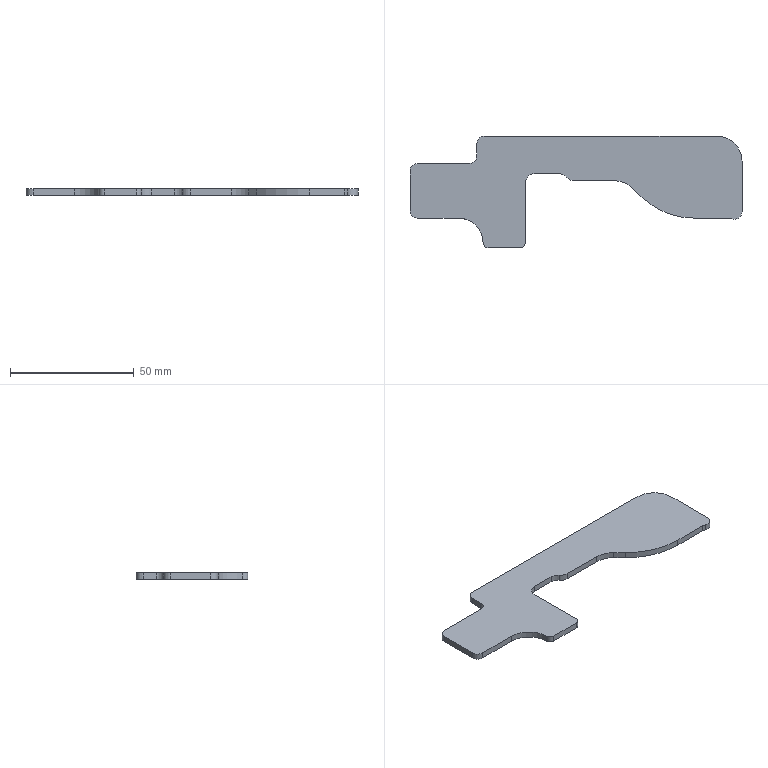Part | STEP file | lll_id338_x_t | 1 solid | 29 faces | box 134 x 45 x 2.5 mm | volume 8850 mm3 | cylinder 15 | plane 14 | commonest cylinder face diameters 6 x6 4 x2 8 x2 20 x2 8.152 x1 20.001 x1
STEP:
#1=CARTESIAN_POINT('',(1078.51,-52.5,0.));
#2=VERTEX_POINT('',#1);
#3=CARTESIAN_POINT('',(1065.5,-52.5,0.));
#4=VERTEX_POINT('',#3);
#5=CARTESIAN_POINT('',(1078.51,-52.5,0.));
#6=DIRECTION('',(-1.,0.,0.));
#7=VECTOR('',#6,1.);
#8=LINE('',#5,#7);
#9=EDGE_CURVE('',#2,#4,#8,.T.);
#10=ORIENTED_EDGE('',*,*,#9,.F.);
#11=CARTESIAN_POINT('',(1078.51,-52.5,2.5));
#12=VERTEX_POINT('',#11);
#13=CARTESIAN_POINT('',(1078.51,-52.5,2.5));
#14=DIRECTION('',(0.,0.,-1.));
#15=VECTOR('',#14,1.);
#16=LINE('',#13,#15);
#17=EDGE_CURVE('',#12,#2,#16,.T.);
#18=ORIENTED_EDGE('',*,*,#17,.F.);
#19=CARTESIAN_POINT('',(1065.5,-52.5,2.5));
#20=VERTEX_POINT('',#19);
#21=CARTESIAN_POINT('',(1078.51,-52.5,2.5));
#22=DIRECTION('',(-1.,0.,0.));
#23=VECTOR('',#22,1.);
#24=LINE('',#21,#23);
#25=EDGE_CURVE('',#12,#20,#24,.T.);
#26=ORIENTED_EDGE('',*,*,#25,.T.);
#27=CARTESIAN_POINT('',(1065.5,-52.5,2.5));
#28=DIRECTION('',(0.,0.,-1.));
#29=VECTOR('',#28,1.);
#30=LINE('',#27,#29);
#31=EDGE_CURVE('',#20,#4,#30,.T.);
#32=ORIENTED_EDGE('',*,*,#31,.T.);
#33=EDGE_LOOP('',(#10,#18,#26,#32));
#34=FACE_OUTER_BOUND('',#33,.T.);
#35=CARTESIAN_POINT('',(1078.51,-52.5,2.5));
#36=DIRECTION('',(0.,-1.,0.));
#37=DIRECTION('',(1.,0.,0.));
#38=AXIS2_PLACEMENT_3D('',#35,#36,#37);
#39=PLANE('',#38);
#40=ADVANCED_FACE('',(#34),#39,.T.);
#41=CARTESIAN_POINT('',(1063.5,-50.5,0.));
#42=VERTEX_POINT('',#41);
#43=CARTESIAN_POINT('',(1065.5,-50.5,0.));
#44=DIRECTION('',(0.,0.,-1.));
#45=DIRECTION('',(1.,0.,0.));
#46=AXIS2_PLACEMENT_3D('',#43,#44,#45);
#47=CIRCLE('',#46,2.);
#48=EDGE_CURVE('',#4,#42,#47,.T.);
#49=ORIENTED_EDGE('',*,*,#48,.F.);
#50=ORIENTED_EDGE('',*,*,#31,.F.);
#51=CARTESIAN_POINT('',(1063.5,-50.5,2.5));
#52=VERTEX_POINT('',#51);
#53=CARTESIAN_POINT('',(1065.5,-50.5,2.5));
#54=DIRECTION('',(0.,0.,-1.));
#55=DIRECTION('',(1.,0.,0.));
#56=AXIS2_PLACEMENT_3D('',#53,#54,#55);
#57=CIRCLE('',#56,2.);
#58=EDGE_CURVE('',#20,#52,#57,.T.);
#59=ORIENTED_EDGE('',*,*,#58,.T.);
#60=CARTESIAN_POINT('',(1063.5,-50.5,2.5));
#61=DIRECTION('',(0.,0.,-1.));
#62=VECTOR('',#61,1.);
#63=LINE('',#60,#62);
#64=EDGE_CURVE('',#52,#42,#63,.T.);
#65=ORIENTED_EDGE('',*,*,#64,.T.);
#66=EDGE_LOOP('',(#49,#50,#59,#65));
#67=FACE_OUTER_BOUND('',#66,.T.);
#68=CARTESIAN_POINT('',(1065.5,-50.5,2.5));
#69=DIRECTION('',(0.,0.,-1.));
#70=DIRECTION('',(-1.,0.,0.));
#71=AXIS2_PLACEMENT_3D('',#68,#69,#70);
#72=CYLINDRICAL_SURFACE('',#71,2.);
#73=ADVANCED_FACE('',(#67),#72,.T.);
#74=CARTESIAN_POINT('',(1053.5,-40.5,0.));
#75=VERTEX_POINT('',#74);
#76=CARTESIAN_POINT('',(1053.499,-50.501,0.));
#77=DIRECTION('',(0.,0.,1.));
#78=DIRECTION('',(1.,0.,0.));
#79=AXIS2_PLACEMENT_3D('',#76,#77,#78);
#80=CIRCLE('',#79,10.001);
#81=EDGE_CURVE('',#42,#75,#80,.T.);
#82=ORIENTED_EDGE('',*,*,#81,.F.);
#83=ORIENTED_EDGE('',*,*,#64,.F.);
#84=CARTESIAN_POINT('',(1053.5,-40.5,2.5));
#85=VERTEX_POINT('',#84);
#86=CARTESIAN_POINT('',(1053.499,-50.501,2.5));
#87=DIRECTION('',(0.,0.,1.));
#88=DIRECTION('',(1.,0.,0.));
#89=AXIS2_PLACEMENT_3D('',#86,#87,#88);
#90=CIRCLE('',#89,10.001);
#91=EDGE_CURVE('',#52,#85,#90,.T.);
#92=ORIENTED_EDGE('',*,*,#91,.T.);
#93=CARTESIAN_POINT('',(1053.5,-40.5,2.5));
#94=DIRECTION('',(0.,0.,-1.));
#95=VECTOR('',#94,1.);
#96=LINE('',#93,#95);
#97=EDGE_CURVE('',#85,#75,#96,.T.);
#98=ORIENTED_EDGE('',*,*,#97,.T.);
#99=EDGE_LOOP('',(#82,#83,#92,#98));
#100=FACE_OUTER_BOUND('',#99,.T.);
#101=CARTESIAN_POINT('',(1053.499,-50.501,2.5));
#102=DIRECTION('',(0.,0.,-1.));
#103=DIRECTION('',(-1.,0.,0.));
#104=AXIS2_PLACEMENT_3D('',#101,#102,#103);
#105=CYLINDRICAL_SURFACE('',#104,10.001);
#106=ADVANCED_FACE('',(#100),#105,.F.);
#107=CARTESIAN_POINT('',(1037.,-40.5,0.));
#108=VERTEX_POINT('',#107);
#109=CARTESIAN_POINT('',(1053.5,-40.5,0.));
#110=DIRECTION('',(-1.,0.,0.));
#111=VECTOR('',#110,1.);
#112=LINE('',#109,#111);
#113=EDGE_CURVE('',#75,#108,#112,.T.);
#114=ORIENTED_EDGE('',*,*,#113,.F.);
#115=ORIENTED_EDGE('',*,*,#97,.F.);
#116=CARTESIAN_POINT('',(1037.,-40.5,2.5));
#117=VERTEX_POINT('',#116);
#118=CARTESIAN_POINT('',(1053.5,-40.5,2.5));
#119=DIRECTION('',(-1.,0.,0.));
#120=VECTOR('',#119,1.);
#121=LINE('',#118,#120);
#122=EDGE_CURVE('',#85,#117,#121,.T.);
#123=ORIENTED_EDGE('',*,*,#122,.T.);
#124=CARTESIAN_POINT('',(1037.,-40.5,2.5));
#125=DIRECTION('',(0.,0.,-1.));
#126=VECTOR('',#125,1.);
#127=LINE('',#124,#126);
#128=EDGE_CURVE('',#117,#108,#127,.T.);
#129=ORIENTED_EDGE('',*,*,#128,.T.);
#130=EDGE_LOOP('',(#114,#115,#123,#129));
#131=FACE_OUTER_BOUND('',#130,.T.);
#132=CARTESIAN_POINT('',(1053.5,-40.5,2.5));
#133=DIRECTION('',(0.,-1.,0.));
#134=DIRECTION('',(1.,0.,0.));
#135=AXIS2_PLACEMENT_3D('',#132,#133,#134);
#136=PLANE('',#135);
#137=ADVANCED_FACE('',(#131),#136,.T.);
#138=CARTESIAN_POINT('',(1034.,-37.5,0.));
#139=VERTEX_POINT('',#138);
#140=CARTESIAN_POINT('',(1037.,-37.5,0.));
#141=DIRECTION('',(0.,0.,-1.));
#142=DIRECTION('',(1.,0.,0.));
#143=AXIS2_PLACEMENT_3D('',#140,#141,#142);
#144=CIRCLE('',#143,3.);
#145=EDGE_CURVE('',#108,#139,#144,.T.);
#146=ORIENTED_EDGE('',*,*,#145,.F.);
#147=ORIENTED_EDGE('',*,*,#128,.F.);
#148=CARTESIAN_POINT('',(1034.,-37.5,2.5));
#149=VERTEX_POINT('',#148);
#150=CARTESIAN_POINT('',(1037.,-37.5,2.5));
#151=DIRECTION('',(0.,0.,-1.));
#152=DIRECTION('',(1.,0.,0.));
#153=AXIS2_PLACEMENT_3D('',#150,#151,#152);
#154=CIRCLE('',#153,3.);
#155=EDGE_CURVE('',#117,#149,#154,.T.);
#156=ORIENTED_EDGE('',*,*,#155,.T.);
#157=CARTESIAN_POINT('',(1034.,-37.5,2.5));
#158=DIRECTION('',(0.,0.,-1.));
#159=VECTOR('',#158,1.);
#160=LINE('',#157,#159);
#161=EDGE_CURVE('',#149,#139,#160,.T.);
#162=ORIENTED_EDGE('',*,*,#161,.T.);
#163=EDGE_LOOP('',(#146,#147,#156,#162));
#164=FACE_OUTER_BOUND('',#163,.T.);
#165=CARTESIAN_POINT('',(1037.,-37.5,2.5));
#166=DIRECTION('',(0.,0.,-1.));
#167=DIRECTION('',(-1.,0.,0.));
#168=AXIS2_PLACEMENT_3D('',#165,#166,#167);
#169=CYLINDRICAL_SURFACE('',#168,3.);
#170=ADVANCED_FACE('',(#164),#169,.T.);
#171=CARTESIAN_POINT('',(1034.,-21.5,0.));
#172=VERTEX_POINT('',#171);
#173=CARTESIAN_POINT('',(1034.,-37.5,0.));
#174=DIRECTION('',(0.,1.,0.));
#175=VECTOR('',#174,1.);
#176=LINE('',#173,#175);
#177=EDGE_CURVE('',#139,#172,#176,.T.);
#178=ORIENTED_EDGE('',*,*,#177,.F.);
#179=ORIENTED_EDGE('',*,*,#161,.F.);
#180=CARTESIAN_POINT('',(1034.,-21.5,2.5));
#181=VERTEX_POINT('',#180);
#182=CARTESIAN_POINT('',(1034.,-37.5,2.5));
#183=DIRECTION('',(0.,1.,0.));
#184=VECTOR('',#183,1.);
#185=LINE('',#182,#184);
#186=EDGE_CURVE('',#149,#181,#185,.T.);
#187=ORIENTED_EDGE('',*,*,#186,.T.);
#188=CARTESIAN_POINT('',(1034.,-21.5,2.5));
#189=DIRECTION('',(0.,0.,-1.));
#190=VECTOR('',#189,1.);
#191=LINE('',#188,#190);
#192=EDGE_CURVE('',#181,#172,#191,.T.);
#193=ORIENTED_EDGE('',*,*,#192,.T.);
#194=EDGE_LOOP('',(#178,#179,#187,#193));
#195=FACE_OUTER_BOUND('',#194,.T.);
#196=CARTESIAN_POINT('',(1034.,-37.5,2.5));
#197=DIRECTION('',(-1.,0.,0.));
#198=DIRECTION('',(0.,0.,1.));
#199=AXIS2_PLACEMENT_3D('',#196,#197,#198);
#200=PLANE('',#199);
#201=ADVANCED_FACE('',(#195),#200,.T.);
#202=CARTESIAN_POINT('',(1037.,-18.5,0.));
#203=VERTEX_POINT('',#202);
#204=CARTESIAN_POINT('',(1037.,-21.5,0.));
#205=DIRECTION('',(0.,0.,-1.));
#206=DIRECTION('',(1.,0.,0.));
#207=AXIS2_PLACEMENT_3D('',#204,#205,#206);
#208=CIRCLE('',#207,3.);
#209=EDGE_CURVE('',#172,#203,#208,.T.);
#210=ORIENTED_EDGE('',*,*,#209,.F.);
#211=ORIENTED_EDGE('',*,*,#192,.F.);
#212=CARTESIAN_POINT('',(1037.,-18.5,2.5));
#213=VERTEX_POINT('',#212);
#214=CARTESIAN_POINT('',(1037.,-21.5,2.5));
#215=DIRECTION('',(0.,0.,-1.));
#216=DIRECTION('',(1.,0.,0.));
#217=AXIS2_PLACEMENT_3D('',#214,#215,#216);
#218=CIRCLE('',#217,3.);
#219=EDGE_CURVE('',#181,#213,#218,.T.);
#220=ORIENTED_EDGE('',*,*,#219,.T.);
#221=CARTESIAN_POINT('',(1037.,-18.5,2.5));
#222=DIRECTION('',(0.,0.,-1.));
#223=VECTOR('',#222,1.);
#224=LINE('',#221,#223);
#225=EDGE_CURVE('',#213,#203,#224,.T.);
#226=ORIENTED_EDGE('',*,*,#225,.T.);
#227=EDGE_LOOP('',(#210,#211,#220,#226));
#228=FACE_OUTER_BOUND('',#227,.T.);
#229=CARTESIAN_POINT('',(1037.,-21.5,2.5));
#230=DIRECTION('',(0.,0.,-1.));
#231=DIRECTION('',(-1.,0.,0.));
#232=AXIS2_PLACEMENT_3D('',#229,#230,#231);
#233=CYLINDRICAL_SURFACE('',#232,3.);
#234=ADVANCED_FACE('',(#228),#233,.T.);
#235=CARTESIAN_POINT('',(1058.,-18.5,0.));
#236=VERTEX_POINT('',#235);
#237=CARTESIAN_POINT('',(1037.,-18.5,0.));
#238=DIRECTION('',(1.,0.,0.));
#239=VECTOR('',#238,1.);
#240=LINE('',#237,#239);
#241=EDGE_CURVE('',#203,#236,#240,.T.);
#242=ORIENTED_EDGE('',*,*,#241,.F.);
#243=ORIENTED_EDGE('',*,*,#225,.F.);
#244=CARTESIAN_POINT('',(1058.,-18.5,2.5));
#245=VERTEX_POINT('',#244);
#246=CARTESIAN_POINT('',(1037.,-18.5,2.5));
#247=DIRECTION('',(1.,0.,0.));
#248=VECTOR('',#247,1.);
#249=LINE('',#246,#248);
#250=EDGE_CURVE('',#213,#245,#249,.T.);
#251=ORIENTED_EDGE('',*,*,#250,.T.);
#252=CARTESIAN_POINT('',(1058.,-18.5,2.5));
#253=DIRECTION('',(0.,0.,-1.));
#254=VECTOR('',#253,1.);
#255=LINE('',#252,#254);
#256=EDGE_CURVE('',#245,#236,#255,.T.);
#257=ORIENTED_EDGE('',*,*,#256,.T.);
#258=EDGE_LOOP('',(#242,#243,#251,#257));
#259=FACE_OUTER_BOUND('',#258,.T.);
#260=CARTESIAN_POINT('',(1037.,-18.5,2.5));
#261=DIRECTION('',(0.,1.,0.));
#262=DIRECTION('',(-1.,0.,0.));
#263=AXIS2_PLACEMENT_3D('',#260,#261,#262);
#264=PLANE('',#263);
#265=ADVANCED_FACE('',(#259),#264,.T.);
#266=CARTESIAN_POINT('',(1061.,-15.5,0.));
#267=VERTEX_POINT('',#266);
#268=CARTESIAN_POINT('',(1058.,-15.5,0.));
#269=DIRECTION('',(0.,0.,1.));
#270=DIRECTION('',(1.,0.,0.));
#271=AXIS2_PLACEMENT_3D('',#268,#269,#270);
#272=CIRCLE('',#271,3.);
#273=EDGE_CURVE('',#236,#267,#272,.T.);
#274=ORIENTED_EDGE('',*,*,#273,.F.);
#275=ORIENTED_EDGE('',*,*,#256,.F.);
#276=CARTESIAN_POINT('',(1061.,-15.5,2.5));
#277=VERTEX_POINT('',#276);
#278=CARTESIAN_POINT('',(1058.,-15.5,2.5));
#279=DIRECTION('',(0.,0.,1.));
#280=DIRECTION('',(1.,0.,0.));
#281=AXIS2_PLACEMENT_3D('',#278,#279,#280);
#282=CIRCLE('',#281,3.);
#283=EDGE_CURVE('',#245,#277,#282,.T.);
#284=ORIENTED_EDGE('',*,*,#283,.T.);
#285=CARTESIAN_POINT('',(1061.,-15.5,2.5));
#286=DIRECTION('',(0.,0.,-1.));
#287=VECTOR('',#286,1.);
#288=LINE('',#285,#287);
#289=EDGE_CURVE('',#277,#267,#288,.T.);
#290=ORIENTED_EDGE('',*,*,#289,.T.);
#291=EDGE_LOOP('',(#274,#275,#284,#290));
#292=FACE_OUTER_BOUND('',#291,.T.);
#293=CARTESIAN_POINT('',(1058.,-15.5,2.5));
#294=DIRECTION('',(0.,0.,-1.));
#295=DIRECTION('',(-1.,0.,0.));
#296=AXIS2_PLACEMENT_3D('',#293,#294,#295);
#297=CYLINDRICAL_SURFACE('',#296,3.);
#298=ADVANCED_FACE('',(#292),#297,.F.);
#299=CARTESIAN_POINT('',(1061.,-10.5,0.));
#300=VERTEX_POINT('',#299);
#301=CARTESIAN_POINT('',(1061.,-15.5,0.));
#302=DIRECTION('',(0.,1.,0.));
#303=VECTOR('',#302,1.);
#304=LINE('',#301,#303);
#305=EDGE_CURVE('',#267,#300,#304,.T.);
#306=ORIENTED_EDGE('',*,*,#305,.F.);
#307=ORIENTED_EDGE('',*,*,#289,.F.);
#308=CARTESIAN_POINT('',(1061.,-10.5,2.5));
#309=VERTEX_POINT('',#308);
#310=CARTESIAN_POINT('',(1061.,-15.5,2.5));
#311=DIRECTION('',(0.,1.,0.));
#312=VECTOR('',#311,1.);
#313=LINE('',#310,#312);
#314=EDGE_CURVE('',#277,#309,#313,.T.);
#315=ORIENTED_EDGE('',*,*,#314,.T.);
#316=CARTESIAN_POINT('',(1061.,-10.5,2.5));
#317=DIRECTION('',(0.,0.,-1.));
#318=VECTOR('',#317,1.);
#319=LINE('',#316,#318);
#320=EDGE_CURVE('',#309,#300,#319,.T.);
#321=ORIENTED_EDGE('',*,*,#320,.T.);
#322=EDGE_LOOP('',(#306,#307,#315,#321));
#323=FACE_OUTER_BOUND('',#322,.T.);
#324=CARTESIAN_POINT('',(1061.,-15.5,2.5));
#325=DIRECTION('',(-1.,0.,0.));
#326=DIRECTION('',(0.,-1.,0.));
#327=AXIS2_PLACEMENT_3D('',#324,#325,#326);
#328=PLANE('',#327);
#329=ADVANCED_FACE('',(#323),#328,.T.);
#330=CARTESIAN_POINT('',(1064.,-7.5,0.));
#331=VERTEX_POINT('',#330);
#332=CARTESIAN_POINT('',(1064.,-10.5,0.));
#333=DIRECTION('',(0.,0.,-1.));
#334=DIRECTION('',(1.,0.,0.));
#335=AXIS2_PLACEMENT_3D('',#332,#333,#334);
#336=CIRCLE('',#335,3.);
#337=EDGE_CURVE('',#300,#331,#336,.T.);
#338=ORIENTED_EDGE('',*,*,#337,.F.);
#339=ORIENTED_EDGE('',*,*,#320,.F.);
#340=CARTESIAN_POINT('',(1064.,-7.5,2.5));
#341=VERTEX_POINT('',#340);
#342=CARTESIAN_POINT('',(1064.,-10.5,2.5));
#343=DIRECTION('',(0.,0.,-1.));
#344=DIRECTION('',(1.,0.,0.));
#345=AXIS2_PLACEMENT_3D('',#342,#343,#344);
#346=CIRCLE('',#345,3.);
#347=EDGE_CURVE('',#309,#341,#346,.T.);
#348=ORIENTED_EDGE('',*,*,#347,.T.);
#349=CARTESIAN_POINT('',(1064.,-7.5,2.5));
#350=DIRECTION('',(0.,0.,-1.));
#351=VECTOR('',#350,1.);
#352=LINE('',#349,#351);
#353=EDGE_CURVE('',#341,#331,#352,.T.);
#354=ORIENTED_EDGE('',*,*,#353,.T.);
#355=EDGE_LOOP('',(#338,#339,#348,#354));
#356=FACE_OUTER_BOUND('',#355,.T.);
#357=CARTESIAN_POINT('',(1064.,-10.5,2.5));
#358=DIRECTION('',(0.,0.,-1.));
#359=DIRECTION('',(-1.,0.,0.));
#360=AXIS2_PLACEMENT_3D('',#357,#358,#359);
#361=CYLINDRICAL_SURFACE('',#360,3.);
#362=ADVANCED_FACE('',(#356),#361,.T.);
#363=CARTESIAN_POINT('',(1158.,-7.5,0.));
#364=VERTEX_POINT('',#363);
#365=CARTESIAN_POINT('',(1064.,-7.5,0.));
#366=DIRECTION('',(1.,0.,0.));
#367=VECTOR('',#366,1.);
#368=LINE('',#365,#367);
#369=EDGE_CURVE('',#331,#364,#368,.T.);
#370=ORIENTED_EDGE('',*,*,#369,.F.);
#371=ORIENTED_EDGE('',*,*,#353,.F.);
#372=CARTESIAN_POINT('',(1158.,-7.5,2.5));
#373=VERTEX_POINT('',#372);
#374=CARTESIAN_POINT('',(1064.,-7.5,2.5));
#375=DIRECTION('',(1.,0.,0.));
#376=VECTOR('',#375,1.);
#377=LINE('',#374,#376);
#378=EDGE_CURVE('',#341,#373,#377,.T.);
#379=ORIENTED_EDGE('',*,*,#378,.T.);
#380=CARTESIAN_POINT('',(1158.,-7.5,2.5));
#381=DIRECTION('',(0.,0.,-1.));
#382=VECTOR('',#381,1.);
#383=LINE('',#380,#382);
#384=EDGE_CURVE('',#373,#364,#383,.T.);
#385=ORIENTED_EDGE('',*,*,#384,.T.);
#386=EDGE_LOOP('',(#370,#371,#379,#385));
#387=FACE_OUTER_BOUND('',#386,.T.);
#388=CARTESIAN_POINT('',(1064.,-7.5,2.5));
#389=DIRECTION('',(0.,1.,0.));
#390=DIRECTION('',(-1.,0.,0.));
#391=AXIS2_PLACEMENT_3D('',#388,#389,#390);
#392=PLANE('',#391);
#393=ADVANCED_FACE('',(#387),#392,.T.);
#394=CARTESIAN_POINT('',(1168.,-17.5,0.));
#395=VERTEX_POINT('',#394);
#396=CARTESIAN_POINT('',(1158.,-17.5,0.));
#397=DIRECTION('',(0.,0.,-1.));
#398=DIRECTION('',(1.,0.,0.));
#399=AXIS2_PLACEMENT_3D('',#396,#397,#398);
#400=CIRCLE('',#399,10.);
#401=EDGE_CURVE('',#364,#395,#400,.T.);
#402=ORIENTED_EDGE('',*,*,#401,.F.);
#403=ORIENTED_EDGE('',*,*,#384,.F.);
#404=CARTESIAN_POINT('',(1168.,-17.5,2.5));
#405=VERTEX_POINT('',#404);
#406=CARTESIAN_POINT('',(1158.,-17.5,2.5));
#407=DIRECTION('',(0.,0.,-1.));
#408=DIRECTION('',(1.,0.,0.));
#409=AXIS2_PLACEMENT_3D('',#406,#407,#408);
#410=CIRCLE('',#409,10.);
#411=EDGE_CURVE('',#373,#405,#410,.T.);
#412=ORIENTED_EDGE('',*,*,#411,.T.);
#413=CARTESIAN_POINT('',(1168.,-17.5,2.5));
#414=DIRECTION('',(0.,0.,-1.));
#415=VECTOR('',#414,1.);
#416=LINE('',#413,#415);
#417=EDGE_CURVE('',#405,#395,#416,.T.);
#418=ORIENTED_EDGE('',*,*,#417,.T.);
#419=EDGE_LOOP('',(#402,#403,#412,#418));
#420=FACE_OUTER_BOUND('',#419,.T.);
#421=CARTESIAN_POINT('',(1158.,-17.5,2.5));
#422=DIRECTION('',(0.,0.,-1.));
#423=DIRECTION('',(-1.,0.,0.));
#424=AXIS2_PLACEMENT_3D('',#421,#422,#423);
#425=CYLINDRICAL_SURFACE('',#424,10.);
#426=ADVANCED_FACE('',(#420),#425,.T.);
#427=CARTESIAN_POINT('',(1168.,-38.,0.));
#428=VERTEX_POINT('',#427);
#429=CARTESIAN_POINT('',(1168.,-17.5,0.));
#430=DIRECTION('',(0.,-1.,0.));
#431=VECTOR('',#430,1.);
#432=LINE('',#429,#431);
#433=EDGE_CURVE('',#395,#428,#432,.T.);
#434=ORIENTED_EDGE('',*,*,#433,.F.);
#435=ORIENTED_EDGE('',*,*,#417,.F.);
#436=CARTESIAN_POINT('',(1168.,-38.,2.5));
#437=VERTEX_POINT('',#436);
#438=CARTESIAN_POINT('',(1168.,-17.5,2.5));
#439=DIRECTION('',(0.,-1.,0.));
#440=VECTOR('',#439,1.);
#441=LINE('',#438,#440);
#442=EDGE_CURVE('',#405,#437,#441,.T.);
#443=ORIENTED_EDGE('',*,*,#442,.T.);
#444=CARTESIAN_POINT('',(1168.,-38.,2.5));
#445=DIRECTION('',(0.,0.,-1.));
#446=VECTOR('',#445,1.);
#447=LINE('',#444,#446);
#448=EDGE_CURVE('',#437,#428,#447,.T.);
#449=ORIENTED_EDGE('',*,*,#448,.T.);
#450=EDGE_LOOP('',(#434,#435,#443,#449));
#451=FACE_OUTER_BOUND('',#450,.T.);
#452=CARTESIAN_POINT('',(1168.,-17.5,2.5));
#453=DIRECTION('',(1.,0.,0.));
#454=DIRECTION('',(0.,1.,0.));
#455=AXIS2_PLACEMENT_3D('',#452,#453,#454);
#456=PLANE('',#455);
#457=ADVANCED_FACE('',(#451),#456,.T.);
#458=CARTESIAN_POINT('',(1163.801,-40.75,0.));
#459=VERTEX_POINT('',#458);
#460=CARTESIAN_POINT('',(1165.,-38.,0.));
#461=DIRECTION('',(0.,0.,-1.));
#462=DIRECTION('',(1.,0.,0.));
#463=AXIS2_PLACEMENT_3D('',#460,#461,#462);
#464=CIRCLE('',#463,3.);
#465=EDGE_CURVE('',#428,#459,#464,.T.);
#466=ORIENTED_EDGE('',*,*,#465,.F.);
#467=ORIENTED_EDGE('',*,*,#448,.F.);
#468=CARTESIAN_POINT('',(1163.801,-40.75,2.5));
#469=VERTEX_POINT('',#468);
#470=CARTESIAN_POINT('',(1165.,-38.,2.5));
#471=DIRECTION('',(0.,0.,-1.));
#472=DIRECTION('',(1.,0.,0.));
#473=AXIS2_PLACEMENT_3D('',#470,#471,#472);
#474=CIRCLE('',#473,3.);
#475=EDGE_CURVE('',#437,#469,#474,.T.);
#476=ORIENTED_EDGE('',*,*,#475,.T.);
#477=CARTESIAN_POINT('',(1163.801,-40.75,2.5));
#478=DIRECTION('',(0.,0.,-1.));
#479=VECTOR('',#478,1.);
#480=LINE('',#477,#479);
#481=EDGE_CURVE('',#469,#459,#480,.T.);
#482=ORIENTED_EDGE('',*,*,#481,.T.);
#483=EDGE_LOOP('',(#466,#467,#476,#482));
#484=FACE_OUTER_BOUND('',#483,.T.);
#485=CARTESIAN_POINT('',(1165.,-38.,2.5));
#486=DIRECTION('',(0.,0.,-1.));
#487=DIRECTION('',(-1.,0.,0.));
#488=AXIS2_PLACEMENT_3D('',#485,#486,#487);
#489=CYLINDRICAL_SURFACE('',#488,3.);
#490=ADVANCED_FACE('',(#484),#489,.T.);
#491=CARTESIAN_POINT('',(1162.602,-40.5,0.));
#492=VERTEX_POINT('',#491);
#493=CARTESIAN_POINT('',(1162.602,-43.5,0.));
#494=DIRECTION('',(0.,0.,1.));
#495=DIRECTION('',(1.,0.,0.));
#496=AXIS2_PLACEMENT_3D('',#493,#494,#495);
#497=CIRCLE('',#496,3.);
#498=EDGE_CURVE('',#459,#492,#497,.T.);
#499=ORIENTED_EDGE('',*,*,#498,.F.);
#500=ORIENTED_EDGE('',*,*,#481,.F.);
#501=CARTESIAN_POINT('',(1162.602,-40.5,2.5));
#502=VERTEX_POINT('',#501);
#503=CARTESIAN_POINT('',(1162.602,-43.5,2.5));
#504=DIRECTION('',(0.,0.,1.));
#505=DIRECTION('',(1.,0.,0.));
#506=AXIS2_PLACEMENT_3D('',#503,#504,#505);
#507=CIRCLE('',#506,3.);
#508=EDGE_CURVE('',#469,#502,#507,.T.);
#509=ORIENTED_EDGE('',*,*,#508,.T.);
#510=CARTESIAN_POINT('',(1162.602,-40.5,2.5));
#511=DIRECTION('',(0.,0.,-1.));
#512=VECTOR('',#511,1.);
#513=LINE('',#510,#512);
#514=EDGE_CURVE('',#502,#492,#513,.T.);
#515=ORIENTED_EDGE('',*,*,#514,.T.);
#516=EDGE_LOOP('',(#499,#500,#509,#515));
#517=FACE_OUTER_BOUND('',#516,.T.);
#518=CARTESIAN_POINT('',(1162.602,-43.5,2.5));
#519=DIRECTION('',(0.,0.,-1.));
#520=DIRECTION('',(-1.,0.,0.));
#521=AXIS2_PLACEMENT_3D('',#518,#519,#520);
#522=CYLINDRICAL_SURFACE('',#521,3.);
#523=ADVANCED_FACE('',(#517),#522,.F.);
#524=CARTESIAN_POINT('',(1148.426,-40.5,0.));
#525=VERTEX_POINT('',#524);
#526=CARTESIAN_POINT('',(1162.602,-40.5,0.));
#527=DIRECTION('',(-1.,0.,0.));
#528=VECTOR('',#527,1.);
#529=LINE('',#526,#528);
#530=EDGE_CURVE('',#492,#525,#529,.T.);
#531=ORIENTED_EDGE('',*,*,#530,.F.);
#532=ORIENTED_EDGE('',*,*,#514,.F.);
#533=CARTESIAN_POINT('',(1148.426,-40.5,2.5));
#534=VERTEX_POINT('',#533);
#535=CARTESIAN_POINT('',(1162.602,-40.5,2.5));
#536=DIRECTION('',(-1.,0.,0.));
#537=VECTOR('',#536,1.);
#538=LINE('',#535,#537);
#539=EDGE_CURVE('',#502,#534,#538,.T.);
#540=ORIENTED_EDGE('',*,*,#539,.T.);
#541=CARTESIAN_POINT('',(1148.426,-40.5,2.5));
#542=DIRECTION('',(0.,0.,-1.));
#543=VECTOR('',#542,1.);
#544=LINE('',#541,#543);
#545=EDGE_CURVE('',#534,#525,#544,.T.);
#546=ORIENTED_EDGE('',*,*,#545,.T.);
#547=EDGE_LOOP('',(#531,#532,#540,#546));
#548=FACE_OUTER_BOUND('',#547,.T.);
#549=CARTESIAN_POINT('',(1162.602,-40.5,2.5));
#550=DIRECTION('',(0.,-1.,0.));
#551=DIRECTION('',(1.,0.,0.));
#552=AXIS2_PLACEMENT_3D('',#549,#550,#551);
#553=PLANE('',#552);
#554=ADVANCED_FACE('',(#548),#553,.T.);
#555=CARTESIAN_POINT('',(1127.213,-31.713,0.));
#556=VERTEX_POINT('',#555);
#557=CARTESIAN_POINT('',(1148.426,-10.502,0.));
#558=DIRECTION('',(0.,0.,-1.));
#559=DIRECTION('',(1.,0.,0.));
#560=AXIS2_PLACEMENT_3D('',#557,#558,#559);
#561=CIRCLE('',#560,29.998);
#562=EDGE_CURVE('',#525,#556,#561,.T.);
#563=ORIENTED_EDGE('',*,*,#562,.F.);
#564=ORIENTED_EDGE('',*,*,#545,.F.);
#565=CARTESIAN_POINT('',(1127.213,-31.713,2.5));
#566=VERTEX_POINT('',#565);
#567=CARTESIAN_POINT('',(1148.426,-10.502,2.5));
#568=DIRECTION('',(0.,0.,-1.));
#569=DIRECTION('',(1.,0.,0.));
#570=AXIS2_PLACEMENT_3D('',#567,#568,#569);
#571=CIRCLE('',#570,29.998);
#572=EDGE_CURVE('',#534,#566,#571,.T.);
#573=ORIENTED_EDGE('',*,*,#572,.T.);
#574=CARTESIAN_POINT('',(1127.213,-31.713,2.5));
#575=DIRECTION('',(0.,0.,-1.));
#576=VECTOR('',#575,1.);
#577=LINE('',#574,#576);
#578=EDGE_CURVE('',#566,#556,#577,.T.);
#579=ORIENTED_EDGE('',*,*,#578,.T.);
#580=EDGE_LOOP('',(#563,#564,#573,#579));
#581=FACE_OUTER_BOUND('',#580,.T.);
#582=CARTESIAN_POINT('',(1148.426,-10.502,2.5));
#583=DIRECTION('',(0.,0.,-1.));
#584=DIRECTION('',(-1.,0.,0.));
#585=AXIS2_PLACEMENT_3D('',#582,#583,#584);
#586=CYLINDRICAL_SURFACE('',#585,29.998);
#587=ADVANCED_FACE('',(#581),#586,.T.);
#588=CARTESIAN_POINT('',(1123.932,-28.432,0.));
#589=VERTEX_POINT('',#588);
#590=CARTESIAN_POINT('',(1127.213,-31.713,0.));
#591=DIRECTION('',(-0.7071,0.7071,0.));
#592=VECTOR('',#591,1.);
#593=LINE('',#590,#592);
#594=EDGE_CURVE('',#556,#589,#593,.T.);
#595=ORIENTED_EDGE('',*,*,#594,.F.);
#596=ORIENTED_EDGE('',*,*,#578,.F.);
#597=CARTESIAN_POINT('',(1123.932,-28.432,2.5));
#598=VERTEX_POINT('',#597);
#599=CARTESIAN_POINT('',(1127.213,-31.713,2.5));
#600=DIRECTION('',(-0.7071,0.7071,0.));
#601=VECTOR('',#600,1.);
#602=LINE('',#599,#601);
#603=EDGE_CURVE('',#566,#598,#602,.T.);
#604=ORIENTED_EDGE('',*,*,#603,.T.);
#605=CARTESIAN_POINT('',(1123.932,-28.432,2.5));
#606=DIRECTION('',(0.,0.,-1.));
#607=VECTOR('',#606,1.);
#608=LINE('',#605,#607);
#609=EDGE_CURVE('',#598,#589,#608,.T.);
#610=ORIENTED_EDGE('',*,*,#609,.T.);
#611=EDGE_LOOP('',(#595,#596,#604,#610));
#612=FACE_OUTER_BOUND('',#611,.T.);
#613=CARTESIAN_POINT('',(1127.213,-31.713,2.5));
#614=DIRECTION('',(-0.7071,-0.7071,0.));
#615=DIRECTION('',(0.7071,-0.7071,0.));
#616=AXIS2_PLACEMENT_3D('',#613,#614,#615);
#617=PLANE('',#616);
#618=ADVANCED_FACE('',(#612),#617,.T.);
#619=CARTESIAN_POINT('',(1116.863,-25.503,0.));
#620=VERTEX_POINT('',#619);
#621=CARTESIAN_POINT('',(1116.86,-35.503,0.));
#622=DIRECTION('',(0.,0.,1.));
#623=DIRECTION('',(1.,0.,0.));
#624=AXIS2_PLACEMENT_3D('',#621,#622,#623);
#625=CIRCLE('',#624,10.);
#626=EDGE_CURVE('',#589,#620,#625,.T.);
#627=ORIENTED_EDGE('',*,*,#626,.F.);
#628=ORIENTED_EDGE('',*,*,#609,.F.);
#629=CARTESIAN_POINT('',(1116.863,-25.503,2.5));
#630=VERTEX_POINT('',#629);
#631=CARTESIAN_POINT('',(1116.86,-35.503,2.5));
#632=DIRECTION('',(0.,0.,1.));
#633=DIRECTION('',(1.,0.,0.));
#634=AXIS2_PLACEMENT_3D('',#631,#632,#633);
#635=CIRCLE('',#634,10.);
#636=EDGE_CURVE('',#598,#630,#635,.T.);
#637=ORIENTED_EDGE('',*,*,#636,.T.);
#638=CARTESIAN_POINT('',(1116.863,-25.503,2.5));
#639=DIRECTION('',(0.,0.,-1.));
#640=VECTOR('',#639,1.);
#641=LINE('',#638,#640);
#642=EDGE_CURVE('',#630,#620,#641,.T.);
#643=ORIENTED_EDGE('',*,*,#642,.T.);
#644=EDGE_LOOP('',(#627,#628,#637,#643));
#645=FACE_OUTER_BOUND('',#644,.T.);
#646=CARTESIAN_POINT('',(1116.86,-35.503,2.5));
#647=DIRECTION('',(0.,0.,-1.));
#648=DIRECTION('',(-1.,0.,0.));
#649=AXIS2_PLACEMENT_3D('',#646,#647,#648);
#650=CYLINDRICAL_SURFACE('',#649,10.);
#651=ADVANCED_FACE('',(#645),#650,.F.);
#652=CARTESIAN_POINT('',(1100.313,-25.498,0.));
#653=VERTEX_POINT('',#652);
#654=CARTESIAN_POINT('',(1116.863,-25.503,0.));
#655=DIRECTION('',(-1.,0.0002888,0.));
#656=VECTOR('',#655,1.);
#657=LINE('',#654,#656);
#658=EDGE_CURVE('',#620,#653,#657,.T.);
#659=ORIENTED_EDGE('',*,*,#658,.F.);
#660=ORIENTED_EDGE('',*,*,#642,.F.);
#661=CARTESIAN_POINT('',(1100.313,-25.498,2.5));
#662=VERTEX_POINT('',#661);
#663=CARTESIAN_POINT('',(1116.863,-25.503,2.5));
#664=DIRECTION('',(-1.,0.0002888,0.));
#665=VECTOR('',#664,1.);
#666=LINE('',#663,#665);
#667=EDGE_CURVE('',#630,#662,#666,.T.);
#668=ORIENTED_EDGE('',*,*,#667,.T.);
#669=CARTESIAN_POINT('',(1100.313,-25.498,2.5));
#670=DIRECTION('',(0.,0.,-1.));
#671=VECTOR('',#670,1.);
#672=LINE('',#669,#671);
#673=EDGE_CURVE('',#662,#653,#672,.T.);
#674=ORIENTED_EDGE('',*,*,#673,.T.);
#675=EDGE_LOOP('',(#659,#660,#668,#674));
#676=FACE_OUTER_BOUND('',#675,.T.);
#677=CARTESIAN_POINT('',(1116.863,-25.503,2.5));
#678=DIRECTION('',(-0.0002888,-1.,0.));
#679=DIRECTION('',(1.,-0.0002888,0.));
#680=AXIS2_PLACEMENT_3D('',#677,#678,#679);
#681=PLANE('',#680);
#682=ADVANCED_FACE('',(#676),#681,.T.);
#683=CARTESIAN_POINT('',(1097.128,-23.983,0.));
#684=VERTEX_POINT('',#683);
#685=CARTESIAN_POINT('',(1100.299,-21.422,0.));
#686=DIRECTION('',(0.,0.,-1.));
#687=DIRECTION('',(1.,0.,0.));
#688=AXIS2_PLACEMENT_3D('',#685,#686,#687);
#689=CIRCLE('',#688,4.076);
#690=EDGE_CURVE('',#653,#684,#689,.T.);
#691=ORIENTED_EDGE('',*,*,#690,.F.);
#692=ORIENTED_EDGE('',*,*,#673,.F.);
#693=CARTESIAN_POINT('',(1097.128,-23.983,2.5));
#694=VERTEX_POINT('',#693);
#695=CARTESIAN_POINT('',(1100.299,-21.422,2.5));
#696=DIRECTION('',(0.,0.,-1.));
#697=DIRECTION('',(1.,0.,0.));
#698=AXIS2_PLACEMENT_3D('',#695,#696,#697);
#699=CIRCLE('',#698,4.076);
#700=EDGE_CURVE('',#662,#694,#699,.T.);
#701=ORIENTED_EDGE('',*,*,#700,.T.);
#702=CARTESIAN_POINT('',(1097.128,-23.983,2.5));
#703=DIRECTION('',(0.,0.,-1.));
#704=VECTOR('',#703,1.);
#705=LINE('',#702,#704);
#706=EDGE_CURVE('',#694,#684,#705,.T.);
#707=ORIENTED_EDGE('',*,*,#706,.T.);
#708=EDGE_LOOP('',(#691,#692,#701,#707));
#709=FACE_OUTER_BOUND('',#708,.T.);
#710=CARTESIAN_POINT('',(1100.299,-21.422,2.5));
#711=DIRECTION('',(0.,0.,-1.));
#712=DIRECTION('',(-1.,0.,0.));
#713=AXIS2_PLACEMENT_3D('',#710,#711,#712);
#714=CYLINDRICAL_SURFACE('',#713,4.076);
#715=ADVANCED_FACE('',(#709),#714,.T.);
#716=CARTESIAN_POINT('',(1094.017,-22.497,0.));
#717=VERTEX_POINT('',#716);
#718=CARTESIAN_POINT('',(1094.016,-26.497,0.));
#719=DIRECTION('',(0.,0.,1.));
#720=DIRECTION('',(1.,0.,0.));
#721=AXIS2_PLACEMENT_3D('',#718,#719,#720);
#722=CIRCLE('',#721,4.);
#723=EDGE_CURVE('',#684,#717,#722,.T.);
#724=ORIENTED_EDGE('',*,*,#723,.F.);
#725=ORIENTED_EDGE('',*,*,#706,.F.);
#726=CARTESIAN_POINT('',(1094.017,-22.497,2.5));
#727=VERTEX_POINT('',#726);
#728=CARTESIAN_POINT('',(1094.016,-26.497,2.5));
#729=DIRECTION('',(0.,0.,1.));
#730=DIRECTION('',(1.,0.,0.));
#731=AXIS2_PLACEMENT_3D('',#728,#729,#730);
#732=CIRCLE('',#731,4.);
#733=EDGE_CURVE('',#694,#727,#732,.T.);
#734=ORIENTED_EDGE('',*,*,#733,.T.);
#735=CARTESIAN_POINT('',(1094.017,-22.497,2.5));
#736=DIRECTION('',(0.,0.,-1.));
#737=VECTOR('',#736,1.);
#738=LINE('',#735,#737);
#739=EDGE_CURVE('',#727,#717,#738,.T.);
#740=ORIENTED_EDGE('',*,*,#739,.T.);
#741=EDGE_LOOP('',(#724,#725,#734,#740));
#742=FACE_OUTER_BOUND('',#741,.T.);
#743=CARTESIAN_POINT('',(1094.016,-26.497,2.5));
#744=DIRECTION('',(0.,0.,-1.));
#745=DIRECTION('',(-1.,0.,0.));
#746=AXIS2_PLACEMENT_3D('',#743,#744,#745);
#747=CYLINDRICAL_SURFACE('',#746,4.);
#748=ADVANCED_FACE('',(#742),#747,.F.);
#749=CARTESIAN_POINT('',(1084.513,-22.495,0.));
#750=VERTEX_POINT('',#749);
#751=CARTESIAN_POINT('',(1094.017,-22.497,0.));
#752=DIRECTION('',(-1.,0.0001728,0.));
#753=VECTOR('',#752,1.);
#754=LINE('',#751,#753);
#755=EDGE_CURVE('',#717,#750,#754,.T.);
#756=ORIENTED_EDGE('',*,*,#755,.F.);
#757=ORIENTED_EDGE('',*,*,#739,.F.);
#758=CARTESIAN_POINT('',(1084.513,-22.495,2.5));
#759=VERTEX_POINT('',#758);
#760=CARTESIAN_POINT('',(1094.017,-22.497,2.5));
#761=DIRECTION('',(-1.,0.0001728,0.));
#762=VECTOR('',#761,1.);
#763=LINE('',#760,#762);
#764=EDGE_CURVE('',#727,#759,#763,.T.);
#765=ORIENTED_EDGE('',*,*,#764,.T.);
#766=CARTESIAN_POINT('',(1084.513,-22.495,2.5));
#767=DIRECTION('',(0.,0.,-1.));
#768=VECTOR('',#767,1.);
#769=LINE('',#766,#768);
#770=EDGE_CURVE('',#759,#750,#769,.T.);
#771=ORIENTED_EDGE('',*,*,#770,.T.);
#772=EDGE_LOOP('',(#756,#757,#765,#771));
#773=FACE_OUTER_BOUND('',#772,.T.);
#774=CARTESIAN_POINT('',(1094.017,-22.497,2.5));
#775=DIRECTION('',(-0.0001728,-1.,0.));
#776=DIRECTION('',(1.,-0.0001728,0.));
#777=AXIS2_PLACEMENT_3D('',#774,#775,#776);
#778=PLANE('',#777);
#779=ADVANCED_FACE('',(#773),#778,.T.);
#780=CARTESIAN_POINT('',(1080.512,-26.495,0.));
#781=VERTEX_POINT('',#780);
#782=CARTESIAN_POINT('',(1084.512,-26.495,0.));
#783=DIRECTION('',(0.,0.,1.));
#784=DIRECTION('',(1.,0.,0.));
#785=AXIS2_PLACEMENT_3D('',#782,#783,#784);
#786=CIRCLE('',#785,4.);
#787=EDGE_CURVE('',#750,#781,#786,.T.);
#788=ORIENTED_EDGE('',*,*,#787,.F.);
#789=ORIENTED_EDGE('',*,*,#770,.F.);
#790=CARTESIAN_POINT('',(1080.512,-26.495,2.5));
#791=VERTEX_POINT('',#790);
#792=CARTESIAN_POINT('',(1084.512,-26.495,2.5));
#793=DIRECTION('',(0.,0.,1.));
#794=DIRECTION('',(1.,0.,0.));
#795=AXIS2_PLACEMENT_3D('',#792,#793,#794);
#796=CIRCLE('',#795,4.);
#797=EDGE_CURVE('',#759,#791,#796,.T.);
#798=ORIENTED_EDGE('',*,*,#797,.T.);
#799=CARTESIAN_POINT('',(1080.512,-26.495,2.5));
#800=DIRECTION('',(0.,0.,-1.));
#801=VECTOR('',#800,1.);
#802=LINE('',#799,#801);
#803=EDGE_CURVE('',#791,#781,#802,.T.);
#804=ORIENTED_EDGE('',*,*,#803,.T.);
#805=EDGE_LOOP('',(#788,#789,#798,#804));
#806=FACE_OUTER_BOUND('',#805,.T.);
#807=CARTESIAN_POINT('',(1084.512,-26.495,2.5));
#808=DIRECTION('',(0.,0.,-1.));
#809=DIRECTION('',(-1.,0.,0.));
#810=AXIS2_PLACEMENT_3D('',#807,#808,#809);
#811=CYLINDRICAL_SURFACE('',#810,4.);
#812=ADVANCED_FACE('',(#806),#811,.F.);
#813=CARTESIAN_POINT('',(1080.51,-50.5,0.));
#814=VERTEX_POINT('',#813);
#815=CARTESIAN_POINT('',(1080.512,-26.495,0.));
#816=DIRECTION('',(-0.00006142,-1.,0.));
#817=VECTOR('',#816,1.);
#818=LINE('',#815,#817);
#819=EDGE_CURVE('',#781,#814,#818,.T.);
#820=ORIENTED_EDGE('',*,*,#819,.F.);
#821=ORIENTED_EDGE('',*,*,#803,.F.);
#822=CARTESIAN_POINT('',(1080.51,-50.5,2.5));
#823=VERTEX_POINT('',#822);
#824=CARTESIAN_POINT('',(1080.512,-26.495,2.5));
#825=DIRECTION('',(-0.00006142,-1.,0.));
#826=VECTOR('',#825,1.);
#827=LINE('',#824,#826);
#828=EDGE_CURVE('',#791,#823,#827,.T.);
#829=ORIENTED_EDGE('',*,*,#828,.T.);
#830=CARTESIAN_POINT('',(1080.51,-50.5,2.5));
#831=DIRECTION('',(0.,0.,-1.));
#832=VECTOR('',#831,1.);
#833=LINE('',#830,#832);
#834=EDGE_CURVE('',#823,#814,#833,.T.);
#835=ORIENTED_EDGE('',*,*,#834,.T.);
#836=EDGE_LOOP('',(#820,#821,#829,#835));
#837=FACE_OUTER_BOUND('',#836,.T.);
#838=CARTESIAN_POINT('',(1080.512,-26.495,2.5));
#839=DIRECTION('',(1.,-0.00006142,0.));
#840=DIRECTION('',(0.00006142,1.,0.));
#841=AXIS2_PLACEMENT_3D('',#838,#839,#840);
#842=PLANE('',#841);
#843=ADVANCED_FACE('',(#837),#842,.T.);
#844=CARTESIAN_POINT('',(1078.51,-50.5,0.));
#845=DIRECTION('',(0.,0.,-1.));
#846=DIRECTION('',(1.,0.,0.));
#847=AXIS2_PLACEMENT_3D('',#844,#845,#846);
#848=CIRCLE('',#847,2.);
#849=EDGE_CURVE('',#814,#2,#848,.T.);
#850=ORIENTED_EDGE('',*,*,#849,.F.);
#851=ORIENTED_EDGE('',*,*,#834,.F.);
#852=CARTESIAN_POINT('',(1078.51,-50.5,2.5));
#853=DIRECTION('',(0.,0.,-1.));
#854=DIRECTION('',(1.,0.,0.));
#855=AXIS2_PLACEMENT_3D('',#852,#853,#854);
#856=CIRCLE('',#855,2.);
#857=EDGE_CURVE('',#823,#12,#856,.T.);
#858=ORIENTED_EDGE('',*,*,#857,.T.);
#859=ORIENTED_EDGE('',*,*,#17,.T.);
#860=EDGE_LOOP('',(#850,#851,#858,#859));
#861=FACE_OUTER_BOUND('',#860,.T.);
#862=CARTESIAN_POINT('',(1078.51,-50.5,2.5));
#863=DIRECTION('',(0.,0.,-1.));
#864=DIRECTION('',(-1.,0.,0.));
#865=AXIS2_PLACEMENT_3D('',#862,#863,#864);
#866=CYLINDRICAL_SURFACE('',#865,2.);
#867=ADVANCED_FACE('',(#861),#866,.T.);
#868=ORIENTED_EDGE('',*,*,#25,.F.);
#869=ORIENTED_EDGE('',*,*,#857,.F.);
#870=ORIENTED_EDGE('',*,*,#828,.F.);
#871=ORIENTED_EDGE('',*,*,#797,.F.);
#872=ORIENTED_EDGE('',*,*,#764,.F.);
#873=ORIENTED_EDGE('',*,*,#733,.F.);
#874=ORIENTED_EDGE('',*,*,#700,.F.);
#875=ORIENTED_EDGE('',*,*,#667,.F.);
#876=ORIENTED_EDGE('',*,*,#636,.F.);
#877=ORIENTED_EDGE('',*,*,#603,.F.);
#878=ORIENTED_EDGE('',*,*,#572,.F.);
#879=ORIENTED_EDGE('',*,*,#539,.F.);
#880=ORIENTED_EDGE('',*,*,#508,.F.);
#881=ORIENTED_EDGE('',*,*,#475,.F.);
#882=ORIENTED_EDGE('',*,*,#442,.F.);
#883=ORIENTED_EDGE('',*,*,#411,.F.);
#884=ORIENTED_EDGE('',*,*,#378,.F.);
#885=ORIENTED_EDGE('',*,*,#347,.F.);
#886=ORIENTED_EDGE('',*,*,#314,.F.);
#887=ORIENTED_EDGE('',*,*,#283,.F.);
#888=ORIENTED_EDGE('',*,*,#250,.F.);
#889=ORIENTED_EDGE('',*,*,#219,.F.);
#890=ORIENTED_EDGE('',*,*,#186,.F.);
#891=ORIENTED_EDGE('',*,*,#155,.F.);
#892=ORIENTED_EDGE('',*,*,#122,.F.);
#893=ORIENTED_EDGE('',*,*,#91,.F.);
#894=ORIENTED_EDGE('',*,*,#58,.F.);
#895=EDGE_LOOP('',(#868,#869,#870,#871,#872,#873,#874,#875,#876,#877,#878,#879,#880,#881,#882,#883,#884,#885,#886,#887,#888,#889,#890,#891,#892,#893,#894));
#896=FACE_OUTER_BOUND('',#895,.T.);
#897=CARTESIAN_POINT('',(1065.5,-50.5,2.5));
#898=DIRECTION('',(0.,0.,-1.));
#899=DIRECTION('',(-1.,0.,0.));
#900=AXIS2_PLACEMENT_3D('',#897,#898,#899);
#901=PLANE('',#900);
#902=ADVANCED_FACE('',(#896),#901,.F.);
#903=ORIENTED_EDGE('',*,*,#9,.T.);
#904=ORIENTED_EDGE('',*,*,#48,.T.);
#905=ORIENTED_EDGE('',*,*,#81,.T.);
#906=ORIENTED_EDGE('',*,*,#113,.T.);
#907=ORIENTED_EDGE('',*,*,#145,.T.);
#908=ORIENTED_EDGE('',*,*,#177,.T.);
#909=ORIENTED_EDGE('',*,*,#209,.T.);
#910=ORIENTED_EDGE('',*,*,#241,.T.);
#911=ORIENTED_EDGE('',*,*,#273,.T.);
#912=ORIENTED_EDGE('',*,*,#305,.T.);
#913=ORIENTED_EDGE('',*,*,#337,.T.);
#914=ORIENTED_EDGE('',*,*,#369,.T.);
#915=ORIENTED_EDGE('',*,*,#401,.T.);
#916=ORIENTED_EDGE('',*,*,#433,.T.);
#917=ORIENTED_EDGE('',*,*,#465,.T.);
#918=ORIENTED_EDGE('',*,*,#498,.T.);
#919=ORIENTED_EDGE('',*,*,#530,.T.);
#920=ORIENTED_EDGE('',*,*,#562,.T.);
#921=ORIENTED_EDGE('',*,*,#594,.T.);
#922=ORIENTED_EDGE('',*,*,#626,.T.);
#923=ORIENTED_EDGE('',*,*,#658,.T.);
#924=ORIENTED_EDGE('',*,*,#690,.T.);
#925=ORIENTED_EDGE('',*,*,#723,.T.);
#926=ORIENTED_EDGE('',*,*,#755,.T.);
#927=ORIENTED_EDGE('',*,*,#787,.T.);
#928=ORIENTED_EDGE('',*,*,#819,.T.);
#929=ORIENTED_EDGE('',*,*,#849,.T.);
#930=EDGE_LOOP('',(#903,#904,#905,#906,#907,#908,#909,#910,#911,#912,#913,#914,#915,#916,#917,#918,#919,#920,#921,#922,#923,#924,#925,#926,#927,#928,#929));
#931=FACE_OUTER_BOUND('',#930,.T.);
#932=CARTESIAN_POINT('',(1065.5,-50.5,0.));
#933=DIRECTION('',(0.,0.,-1.));
#934=DIRECTION('',(-1.,0.,0.));
#935=AXIS2_PLACEMENT_3D('',#932,#933,#934);
#936=PLANE('',#935);
#937=ADVANCED_FACE('',(#931),#936,.T.);
#938=CLOSED_SHELL('',(#40,#73,#106,#137,#170,#201,#234,#265,#298,#329,#362,#393,#426,#457,#490,#523,#554,#587,#618,#651,#682,#715,#748,#779,#812,#843,#867,#902,#937));
#939=MANIFOLD_SOLID_BREP('',#938);
#940=(LENGTH_UNIT()NAMED_UNIT(*)SI_UNIT(.MILLI.,.METRE.));
#941=UNCERTAINTY_MEASURE_WITH_UNIT(LENGTH_MEASURE(0.00002),#940,'','');
#942=(NAMED_UNIT(*)PLANE_ANGLE_UNIT()SI_UNIT($,.RADIAN.));
#943=PLANE_ANGLE_MEASURE_WITH_UNIT(PLANE_ANGLE_MEASURE(0.01745),#942);
#944=DIMENSIONAL_EXPONENTS(0.,0.,0.,0.,0.,0.,0.);
#945=(CONVERSION_BASED_UNIT('DEGREE',#943)NAMED_UNIT(#944)PLANE_ANGLE_UNIT());
#946=(NAMED_UNIT(*)SI_UNIT($,.STERADIAN.)SOLID_ANGLE_UNIT());
#947=(GEOMETRIC_REPRESENTATION_CONTEXT(3)GLOBAL_UNCERTAINTY_ASSIGNED_CONTEXT((#941))GLOBAL_UNIT_ASSIGNED_CONTEXT((#940,#945,#946))REPRESENTATION_CONTEXT('',''));
#948=ADVANCED_BREP_SHAPE_REPRESENTATION('',(#939),#947);